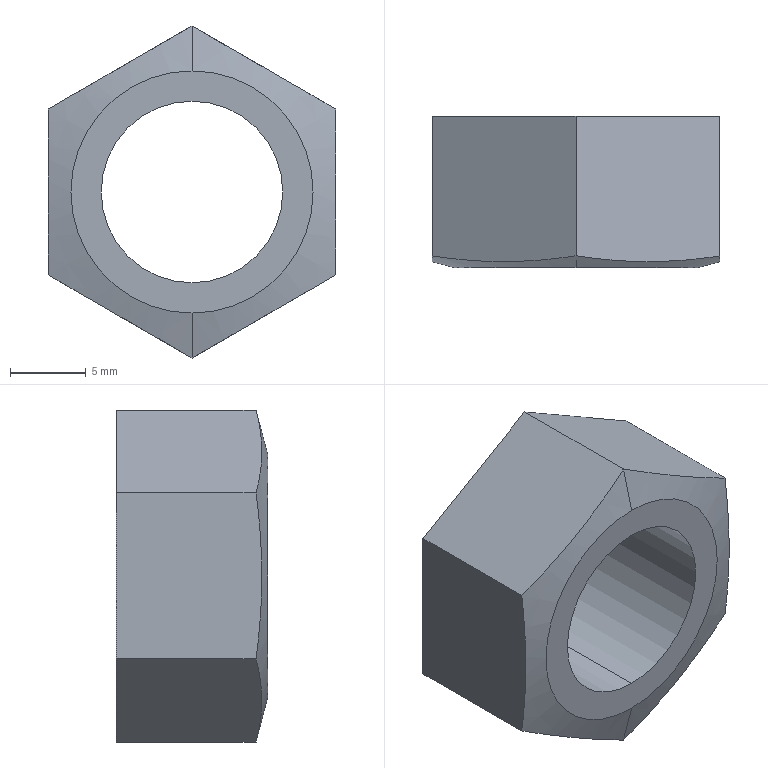Part | STEP file | FJSM12nut | 1 solid | 12 faces | box 19 x 10 x 21.939 mm | volume 1964 mm3 | plane 8 | cone 2 | cylinder 2 | commonest cylinder face diameters 12 x2
STEP:
#1=CARTESIAN_POINT('',(0.,0.,8.));
#2=VERTEX_POINT('',#1);
#3=CARTESIAN_POINT('',(0.,0.,-8.));
#4=VERTEX_POINT('',#3);
#5=CARTESIAN_POINT('',(0.,0.,0.));
#6=DIRECTION('',(0.,1.,0.));
#7=DIRECTION('',(0.,0.,1.));
#8=AXIS2_PLACEMENT_3D('',#5,#6,#7);
#9=CIRCLE('',#8,8.);
#10=EDGE_CURVE('',#2,#4,#9,.T.);
#11=ORIENTED_EDGE('',*,*,#10,.T.);
#12=CARTESIAN_POINT('',(0.,0.7664,-10.97));
#13=VERTEX_POINT('',#12);
#14=CARTESIAN_POINT('',(0.,0.,-8.));
#15=DIRECTION('',(0.,0.2499,-0.9683));
#16=VECTOR('',#15,1000.);
#17=LINE('',#14,#16);
#18=EDGE_CURVE('',#4,#13,#17,.T.);
#19=ORIENTED_EDGE('',*,*,#18,.T.);
#20=CARTESIAN_POINT('',(9.5,0.7664,-5.485));
#21=VERTEX_POINT('',#20);
#22=CARTESIAN_POINT('',(0.,0.7664,-10.97));
#23=CARTESIAN_POINT('',(0.7917,0.6484,-10.513));
#24=CARTESIAN_POINT('',(1.583,0.5526,-10.056));
#25=CARTESIAN_POINT('',(3.167,0.4218,-9.141));
#26=CARTESIAN_POINT('',(4.75,0.3524,-8.227));
#27=CARTESIAN_POINT('',(6.333,0.4218,-7.313));
#28=CARTESIAN_POINT('',(7.917,0.5526,-6.399));
#29=CARTESIAN_POINT('',(8.708,0.6484,-5.942));
#30=CARTESIAN_POINT('',(9.5,0.7664,-5.485));
#31=B_SPLINE_CURVE_WITH_KNOTS('',3,(#22,#23,#24,#25,#26,#27,#28,#29,#30),.UNSPECIFIED.,.F.,.F.,(4,2,1,2,4),(0.000000231,0.002743,0.005485,0.008227,0.01097),.UNSPECIFIED.);
#32=EDGE_CURVE('',#13,#21,#31,.T.);
#33=ORIENTED_EDGE('',*,*,#32,.T.);
#34=CARTESIAN_POINT('',(9.5,0.7664,5.485));
#35=VERTEX_POINT('',#34);
#36=CARTESIAN_POINT('',(9.5,0.7664,-5.485));
#37=CARTESIAN_POINT('',(9.5,0.6486,-4.572));
#38=CARTESIAN_POINT('',(9.5,0.5523,-3.654));
#39=CARTESIAN_POINT('',(9.5,0.4214,-1.821));
#40=CARTESIAN_POINT('',(9.5,0.3869,-0.9056));
#41=CARTESIAN_POINT('',(9.5,0.3873,0.9233));
#42=CARTESIAN_POINT('',(9.5,0.4222,1.837));
#43=CARTESIAN_POINT('',(9.5,0.5532,3.662));
#44=CARTESIAN_POINT('',(9.5,0.6488,4.574));
#45=CARTESIAN_POINT('',(9.5,0.7664,5.485));
#46=B_SPLINE_CURVE_WITH_KNOTS('',3,(#36,#37,#38,#39,#40,#41,#42,#43,#44,#45),.UNSPECIFIED.,.F.,.F.,(4,2,2,2,4),(0.009151,0.01191,0.01467,0.01743,0.02019),.UNSPECIFIED.);
#47=EDGE_CURVE('',#21,#35,#46,.T.);
#48=ORIENTED_EDGE('',*,*,#47,.T.);
#49=CARTESIAN_POINT('',(0.,0.7664,10.97));
#50=VERTEX_POINT('',#49);
#51=CARTESIAN_POINT('',(9.5,0.7664,5.485));
#52=CARTESIAN_POINT('',(8.708,0.6484,5.942));
#53=CARTESIAN_POINT('',(7.917,0.5526,6.399));
#54=CARTESIAN_POINT('',(6.333,0.4218,7.313));
#55=CARTESIAN_POINT('',(4.75,0.3524,8.227));
#56=CARTESIAN_POINT('',(3.167,0.4218,9.141));
#57=CARTESIAN_POINT('',(1.583,0.5526,10.056));
#58=CARTESIAN_POINT('',(0.7917,0.6484,10.513));
#59=CARTESIAN_POINT('',(0.,0.7664,10.97));
#60=B_SPLINE_CURVE_WITH_KNOTS('',3,(#51,#52,#53,#54,#55,#56,#57,#58,#59),.UNSPECIFIED.,.F.,.F.,(4,2,1,2,4),(0.000000231,0.002743,0.005485,0.008227,0.01097),.UNSPECIFIED.);
#61=EDGE_CURVE('',#35,#50,#60,.T.);
#62=ORIENTED_EDGE('',*,*,#61,.T.);
#63=CARTESIAN_POINT('',(0.,0.,8.));
#64=DIRECTION('',(0.,0.2499,0.9683));
#65=VECTOR('',#64,1000.);
#66=LINE('',#63,#65);
#67=EDGE_CURVE('',#2,#50,#66,.T.);
#68=ORIENTED_EDGE('',*,*,#67,.F.);
#69=EDGE_LOOP('',(#11,#19,#33,#48,#62,#68));
#70=FACE_OUTER_BOUND('',#69,.T.);
#71=CARTESIAN_POINT('',(0.,0.,0.));
#72=DIRECTION('',(0.,1.,0.));
#73=DIRECTION('',(0.,0.,1.));
#74=AXIS2_PLACEMENT_3D('',#71,#72,#73);
#75=CONICAL_SURFACE('',#74,8.,1.318);
#76=ADVANCED_FACE('',(#70),#75,.T.);
#77=CARTESIAN_POINT('',(0.,0.,-6.));
#78=VERTEX_POINT('',#77);
#79=CARTESIAN_POINT('',(0.,0.,6.));
#80=VERTEX_POINT('',#79);
#81=CARTESIAN_POINT('',(0.,0.,0.));
#82=DIRECTION('',(0.,1.,0.));
#83=DIRECTION('',(0.,0.,1.));
#84=AXIS2_PLACEMENT_3D('',#81,#82,#83);
#85=CIRCLE('',#84,6.);
#86=EDGE_CURVE('',#78,#80,#85,.T.);
#87=ORIENTED_EDGE('',*,*,#86,.F.);
#88=CARTESIAN_POINT('',(0.,10.,-6.));
#89=VERTEX_POINT('',#88);
#90=CARTESIAN_POINT('',(0.,0.,-6.));
#91=DIRECTION('',(0.,1.,0.));
#92=VECTOR('',#91,1000.);
#93=LINE('',#90,#92);
#94=EDGE_CURVE('',#78,#89,#93,.T.);
#95=ORIENTED_EDGE('',*,*,#94,.T.);
#96=CARTESIAN_POINT('',(0.,10.,6.));
#97=VERTEX_POINT('',#96);
#98=CARTESIAN_POINT('',(0.,10.,0.));
#99=DIRECTION('',(0.,1.,0.));
#100=DIRECTION('',(0.,0.,1.));
#101=AXIS2_PLACEMENT_3D('',#98,#99,#100);
#102=CIRCLE('',#101,6.);
#103=EDGE_CURVE('',#89,#97,#102,.T.);
#104=ORIENTED_EDGE('',*,*,#103,.T.);
#105=CARTESIAN_POINT('',(0.,0.,6.));
#106=DIRECTION('',(0.,1.,0.));
#107=VECTOR('',#106,1000.);
#108=LINE('',#105,#107);
#109=EDGE_CURVE('',#80,#97,#108,.T.);
#110=ORIENTED_EDGE('',*,*,#109,.F.);
#111=EDGE_LOOP('',(#87,#95,#104,#110));
#112=FACE_OUTER_BOUND('',#111,.T.);
#113=CARTESIAN_POINT('',(0.,0.,0.));
#114=DIRECTION('',(0.,1.,0.));
#115=DIRECTION('',(0.,0.,1.));
#116=AXIS2_PLACEMENT_3D('',#113,#114,#115);
#117=CYLINDRICAL_SURFACE('',#116,6.);
#118=ADVANCED_FACE('',(#112),#117,.F.);
#119=ORIENTED_EDGE('',*,*,#94,.F.);
#120=CARTESIAN_POINT('',(0.,0.,0.));
#121=DIRECTION('',(0.,1.,0.));
#122=DIRECTION('',(0.,0.,1.));
#123=AXIS2_PLACEMENT_3D('',#120,#121,#122);
#124=CIRCLE('',#123,6.);
#125=EDGE_CURVE('',#80,#78,#124,.T.);
#126=ORIENTED_EDGE('',*,*,#125,.F.);
#127=ORIENTED_EDGE('',*,*,#109,.T.);
#128=CARTESIAN_POINT('',(0.,10.,0.));
#129=DIRECTION('',(0.,1.,0.));
#130=DIRECTION('',(0.,0.,1.));
#131=AXIS2_PLACEMENT_3D('',#128,#129,#130);
#132=CIRCLE('',#131,6.);
#133=EDGE_CURVE('',#97,#89,#132,.T.);
#134=ORIENTED_EDGE('',*,*,#133,.T.);
#135=EDGE_LOOP('',(#119,#126,#127,#134));
#136=FACE_OUTER_BOUND('',#135,.T.);
#137=CARTESIAN_POINT('',(0.,0.,0.));
#138=DIRECTION('',(0.,1.,0.));
#139=DIRECTION('',(0.,0.,1.));
#140=AXIS2_PLACEMENT_3D('',#137,#138,#139);
#141=CYLINDRICAL_SURFACE('',#140,6.);
#142=ADVANCED_FACE('',(#136),#141,.F.);
#143=ORIENTED_EDGE('',*,*,#10,.F.);
#144=CARTESIAN_POINT('',(0.,0.,0.));
#145=DIRECTION('',(0.,1.,0.));
#146=DIRECTION('',(0.,0.,1.));
#147=AXIS2_PLACEMENT_3D('',#144,#145,#146);
#148=CIRCLE('',#147,8.);
#149=EDGE_CURVE('',#4,#2,#148,.T.);
#150=ORIENTED_EDGE('',*,*,#149,.F.);
#151=EDGE_LOOP('',(#143,#150));
#152=FACE_OUTER_BOUND('',#151,.T.);
#153=ORIENTED_EDGE('',*,*,#125,.T.);
#154=ORIENTED_EDGE('',*,*,#86,.T.);
#155=EDGE_LOOP('',(#153,#154));
#156=FACE_BOUND('',#155,.T.);
#157=CARTESIAN_POINT('',(6.,0.,0.));
#158=DIRECTION('',(0.,1.,0.));
#159=DIRECTION('',(0.,0.,1.));
#160=AXIS2_PLACEMENT_3D('',#157,#158,#159);
#161=PLANE('',#160);
#162=ADVANCED_FACE('',(#152,#156),#161,.F.);
#163=ORIENTED_EDGE('',*,*,#18,.F.);
#164=ORIENTED_EDGE('',*,*,#149,.T.);
#165=ORIENTED_EDGE('',*,*,#67,.T.);
#166=CARTESIAN_POINT('',(-9.5,0.7664,5.485));
#167=VERTEX_POINT('',#166);
#168=CARTESIAN_POINT('',(0.,0.7664,10.97));
#169=CARTESIAN_POINT('',(-0.7917,0.6484,10.513));
#170=CARTESIAN_POINT('',(-1.583,0.5526,10.056));
#171=CARTESIAN_POINT('',(-3.167,0.4218,9.141));
#172=CARTESIAN_POINT('',(-4.75,0.3524,8.227));
#173=CARTESIAN_POINT('',(-6.333,0.4218,7.313));
#174=CARTESIAN_POINT('',(-7.917,0.5526,6.399));
#175=CARTESIAN_POINT('',(-8.708,0.6484,5.942));
#176=CARTESIAN_POINT('',(-9.5,0.7664,5.485));
#177=B_SPLINE_CURVE_WITH_KNOTS('',3,(#168,#169,#170,#171,#172,#173,#174,#175,#176),.UNSPECIFIED.,.F.,.F.,(4,2,1,2,4),(0.000000231,0.002743,0.005485,0.008227,0.01097),.UNSPECIFIED.);
#178=EDGE_CURVE('',#50,#167,#177,.T.);
#179=ORIENTED_EDGE('',*,*,#178,.T.);
#180=CARTESIAN_POINT('',(-9.5,0.7664,-5.485));
#181=VERTEX_POINT('',#180);
#182=CARTESIAN_POINT('',(-9.5,0.7664,5.485));
#183=CARTESIAN_POINT('',(-9.5,0.6488,4.574));
#184=CARTESIAN_POINT('',(-9.5,0.5532,3.662));
#185=CARTESIAN_POINT('',(-9.5,0.4222,1.837));
#186=CARTESIAN_POINT('',(-9.5,0.3873,0.9233));
#187=CARTESIAN_POINT('',(-9.5,0.3869,-0.9056));
#188=CARTESIAN_POINT('',(-9.5,0.4214,-1.821));
#189=CARTESIAN_POINT('',(-9.5,0.5523,-3.654));
#190=CARTESIAN_POINT('',(-9.5,0.6486,-4.572));
#191=CARTESIAN_POINT('',(-9.5,0.7664,-5.485));
#192=B_SPLINE_CURVE_WITH_KNOTS('',3,(#182,#183,#184,#185,#186,#187,#188,#189,#190,#191),.UNSPECIFIED.,.F.,.F.,(4,2,2,2,4),(0.02104,0.02379,0.02655,0.0293,0.03206),.UNSPECIFIED.);
#193=EDGE_CURVE('',#167,#181,#192,.T.);
#194=ORIENTED_EDGE('',*,*,#193,.T.);
#195=CARTESIAN_POINT('',(-9.5,0.7664,-5.485));
#196=CARTESIAN_POINT('',(-8.708,0.6484,-5.942));
#197=CARTESIAN_POINT('',(-7.917,0.5526,-6.399));
#198=CARTESIAN_POINT('',(-6.333,0.4218,-7.313));
#199=CARTESIAN_POINT('',(-4.75,0.3524,-8.227));
#200=CARTESIAN_POINT('',(-3.167,0.4218,-9.141));
#201=CARTESIAN_POINT('',(-1.583,0.5526,-10.056));
#202=CARTESIAN_POINT('',(-0.7917,0.6484,-10.513));
#203=CARTESIAN_POINT('',(0.,0.7664,-10.97));
#204=B_SPLINE_CURVE_WITH_KNOTS('',3,(#195,#196,#197,#198,#199,#200,#201,#202,#203),.UNSPECIFIED.,.F.,.F.,(4,2,1,2,4),(0.000000231,0.002743,0.005485,0.008227,0.01097),.UNSPECIFIED.);
#205=EDGE_CURVE('',#181,#13,#204,.T.);
#206=ORIENTED_EDGE('',*,*,#205,.T.);
#207=EDGE_LOOP('',(#163,#164,#165,#179,#194,#206));
#208=FACE_OUTER_BOUND('',#207,.T.);
#209=CARTESIAN_POINT('',(0.,0.,0.));
#210=DIRECTION('',(0.,1.,0.));
#211=DIRECTION('',(0.,0.,1.));
#212=AXIS2_PLACEMENT_3D('',#209,#210,#211);
#213=CONICAL_SURFACE('',#212,8.,1.318);
#214=ADVANCED_FACE('',(#208),#213,.T.);
#215=CARTESIAN_POINT('',(9.5,10.,-5.485));
#216=VERTEX_POINT('',#215);
#217=CARTESIAN_POINT('',(0.,10.,-10.97));
#218=VERTEX_POINT('',#217);
#219=CARTESIAN_POINT('',(13.656,10.,-3.085));
#220=DIRECTION('',(-0.866,0.,-0.5));
#221=VECTOR('',#220,1000.);
#222=LINE('',#219,#221);
#223=EDGE_CURVE('',#216,#218,#222,.T.);
#224=ORIENTED_EDGE('',*,*,#223,.T.);
#225=CARTESIAN_POINT('',(-9.5,10.,-5.485));
#226=VERTEX_POINT('',#225);
#227=CARTESIAN_POINT('',(4.156,10.,-13.369));
#228=DIRECTION('',(-0.866,0.,0.5));
#229=VECTOR('',#228,1000.);
#230=LINE('',#227,#229);
#231=EDGE_CURVE('',#218,#226,#230,.T.);
#232=ORIENTED_EDGE('',*,*,#231,.T.);
#233=CARTESIAN_POINT('',(-9.5,10.,5.485));
#234=VERTEX_POINT('',#233);
#235=CARTESIAN_POINT('',(-9.5,10.,0.));
#236=DIRECTION('',(0.,0.,1.));
#237=VECTOR('',#236,1000.);
#238=LINE('',#235,#237);
#239=EDGE_CURVE('',#226,#234,#238,.T.);
#240=ORIENTED_EDGE('',*,*,#239,.T.);
#241=CARTESIAN_POINT('',(0.,10.,10.97));
#242=VERTEX_POINT('',#241);
#243=CARTESIAN_POINT('',(4.156,10.,13.369));
#244=DIRECTION('',(0.866,0.,0.5));
#245=VECTOR('',#244,1000.);
#246=LINE('',#243,#245);
#247=EDGE_CURVE('',#234,#242,#246,.T.);
#248=ORIENTED_EDGE('',*,*,#247,.T.);
#249=CARTESIAN_POINT('',(9.5,10.,5.485));
#250=VERTEX_POINT('',#249);
#251=CARTESIAN_POINT('',(13.656,10.,3.085));
#252=DIRECTION('',(0.866,0.,-0.5));
#253=VECTOR('',#252,1000.);
#254=LINE('',#251,#253);
#255=EDGE_CURVE('',#242,#250,#254,.T.);
#256=ORIENTED_EDGE('',*,*,#255,.T.);
#257=CARTESIAN_POINT('',(9.5,10.,0.));
#258=DIRECTION('',(0.,0.,-1.));
#259=VECTOR('',#258,1000.);
#260=LINE('',#257,#259);
#261=EDGE_CURVE('',#250,#216,#260,.T.);
#262=ORIENTED_EDGE('',*,*,#261,.T.);
#263=EDGE_LOOP('',(#224,#232,#240,#248,#256,#262));
#264=FACE_OUTER_BOUND('',#263,.T.);
#265=ORIENTED_EDGE('',*,*,#133,.F.);
#266=ORIENTED_EDGE('',*,*,#103,.F.);
#267=EDGE_LOOP('',(#265,#266));
#268=FACE_BOUND('',#267,.T.);
#269=CARTESIAN_POINT('',(11.875,10.,0.));
#270=DIRECTION('',(0.,-1.,0.));
#271=DIRECTION('',(0.,0.,-1.));
#272=AXIS2_PLACEMENT_3D('',#269,#270,#271);
#273=PLANE('',#272);
#274=ADVANCED_FACE('',(#264,#268),#273,.F.);
#275=CARTESIAN_POINT('',(-9.5,11.,-5.485));
#276=DIRECTION('',(0.,-1.,0.));
#277=VECTOR('',#276,1000.);
#278=LINE('',#275,#277);
#279=EDGE_CURVE('',#226,#181,#278,.T.);
#280=ORIENTED_EDGE('',*,*,#279,.F.);
#281=ORIENTED_EDGE('',*,*,#231,.F.);
#282=CARTESIAN_POINT('',(0.,11.,-10.97));
#283=DIRECTION('',(0.,-1.,0.));
#284=VECTOR('',#283,1000.);
#285=LINE('',#282,#284);
#286=EDGE_CURVE('',#218,#13,#285,.T.);
#287=ORIENTED_EDGE('',*,*,#286,.T.);
#288=ORIENTED_EDGE('',*,*,#205,.F.);
#289=EDGE_LOOP('',(#280,#281,#287,#288));
#290=FACE_OUTER_BOUND('',#289,.T.);
#291=CARTESIAN_POINT('',(0.,11.,-10.97));
#292=DIRECTION('',(0.5,0.,0.866));
#293=DIRECTION('',(0.866,0.,-0.5));
#294=AXIS2_PLACEMENT_3D('',#291,#292,#293);
#295=PLANE('',#294);
#296=ADVANCED_FACE('',(#290),#295,.F.);
#297=CARTESIAN_POINT('',(-9.5,11.,5.485));
#298=DIRECTION('',(0.,-1.,0.));
#299=VECTOR('',#298,1000.);
#300=LINE('',#297,#299);
#301=EDGE_CURVE('',#234,#167,#300,.T.);
#302=ORIENTED_EDGE('',*,*,#301,.F.);
#303=ORIENTED_EDGE('',*,*,#239,.F.);
#304=ORIENTED_EDGE('',*,*,#279,.T.);
#305=ORIENTED_EDGE('',*,*,#193,.F.);
#306=EDGE_LOOP('',(#302,#303,#304,#305));
#307=FACE_OUTER_BOUND('',#306,.T.);
#308=CARTESIAN_POINT('',(-9.5,11.,-5.485));
#309=DIRECTION('',(1.,0.,0.));
#310=DIRECTION('',(0.,0.,-1.));
#311=AXIS2_PLACEMENT_3D('',#308,#309,#310);
#312=PLANE('',#311);
#313=ADVANCED_FACE('',(#307),#312,.F.);
#314=CARTESIAN_POINT('',(0.,11.,10.97));
#315=DIRECTION('',(0.,-1.,0.));
#316=VECTOR('',#315,1000.);
#317=LINE('',#314,#316);
#318=EDGE_CURVE('',#242,#50,#317,.T.);
#319=ORIENTED_EDGE('',*,*,#318,.F.);
#320=ORIENTED_EDGE('',*,*,#247,.F.);
#321=ORIENTED_EDGE('',*,*,#301,.T.);
#322=ORIENTED_EDGE('',*,*,#178,.F.);
#323=EDGE_LOOP('',(#319,#320,#321,#322));
#324=FACE_OUTER_BOUND('',#323,.T.);
#325=CARTESIAN_POINT('',(-9.5,11.,5.485));
#326=DIRECTION('',(0.5,0.,-0.866));
#327=DIRECTION('',(-0.866,0.,-0.5));
#328=AXIS2_PLACEMENT_3D('',#325,#326,#327);
#329=PLANE('',#328);
#330=ADVANCED_FACE('',(#324),#329,.F.);
#331=CARTESIAN_POINT('',(9.5,11.,5.485));
#332=DIRECTION('',(0.,-1.,0.));
#333=VECTOR('',#332,1000.);
#334=LINE('',#331,#333);
#335=EDGE_CURVE('',#250,#35,#334,.T.);
#336=ORIENTED_EDGE('',*,*,#335,.F.);
#337=ORIENTED_EDGE('',*,*,#255,.F.);
#338=ORIENTED_EDGE('',*,*,#318,.T.);
#339=ORIENTED_EDGE('',*,*,#61,.F.);
#340=EDGE_LOOP('',(#336,#337,#338,#339));
#341=FACE_OUTER_BOUND('',#340,.T.);
#342=CARTESIAN_POINT('',(0.,11.,10.97));
#343=DIRECTION('',(-0.5,0.,-0.866));
#344=DIRECTION('',(-0.866,0.,0.5));
#345=AXIS2_PLACEMENT_3D('',#342,#343,#344);
#346=PLANE('',#345);
#347=ADVANCED_FACE('',(#341),#346,.F.);
#348=CARTESIAN_POINT('',(9.5,11.,-5.485));
#349=DIRECTION('',(0.,-1.,0.));
#350=VECTOR('',#349,1000.);
#351=LINE('',#348,#350);
#352=EDGE_CURVE('',#216,#21,#351,.T.);
#353=ORIENTED_EDGE('',*,*,#352,.F.);
#354=ORIENTED_EDGE('',*,*,#261,.F.);
#355=ORIENTED_EDGE('',*,*,#335,.T.);
#356=ORIENTED_EDGE('',*,*,#47,.F.);
#357=EDGE_LOOP('',(#353,#354,#355,#356));
#358=FACE_OUTER_BOUND('',#357,.T.);
#359=CARTESIAN_POINT('',(9.5,11.,5.485));
#360=DIRECTION('',(-1.,0.,0.));
#361=DIRECTION('',(0.,0.,1.));
#362=AXIS2_PLACEMENT_3D('',#359,#360,#361);
#363=PLANE('',#362);
#364=ADVANCED_FACE('',(#358),#363,.F.);
#365=ORIENTED_EDGE('',*,*,#286,.F.);
#366=ORIENTED_EDGE('',*,*,#223,.F.);
#367=ORIENTED_EDGE('',*,*,#352,.T.);
#368=ORIENTED_EDGE('',*,*,#32,.F.);
#369=EDGE_LOOP('',(#365,#366,#367,#368));
#370=FACE_OUTER_BOUND('',#369,.T.);
#371=CARTESIAN_POINT('',(9.5,11.,-5.485));
#372=DIRECTION('',(-0.5,0.,0.866));
#373=DIRECTION('',(0.866,0.,0.5));
#374=AXIS2_PLACEMENT_3D('',#371,#372,#373);
#375=PLANE('',#374);
#376=ADVANCED_FACE('',(#370),#375,.F.);
#377=CLOSED_SHELL('',(#76,#118,#142,#162,#214,#274,#296,#313,#330,#347,#364,#376));
#378=MANIFOLD_SOLID_BREP('',#377);
#379=CARTESIAN_POINT('',(0.,0.,0.));
#380=DIRECTION('',(0.,0.,1.));
#381=DIRECTION('',(1.,0.,0.));
#382=AXIS2_PLACEMENT_3D('',#379,#380,#381);
#383=(LENGTH_UNIT()NAMED_UNIT(*)SI_UNIT(.MILLI.,.METRE.));
#384=UNCERTAINTY_MEASURE_WITH_UNIT(LENGTH_MEASURE(0.00001),#383,'','');
#385=(NAMED_UNIT(*)PLANE_ANGLE_UNIT()SI_UNIT($,.RADIAN.));
#386=(NAMED_UNIT(*)SI_UNIT($,.STERADIAN.)SOLID_ANGLE_UNIT());
#387=(GEOMETRIC_REPRESENTATION_CONTEXT(3)GLOBAL_UNCERTAINTY_ASSIGNED_CONTEXT((#384))GLOBAL_UNIT_ASSIGNED_CONTEXT((#383,#385,#386))REPRESENTATION_CONTEXT('',''));
#388=ADVANCED_BREP_SHAPE_REPRESENTATION('',(#378,#382),#387);